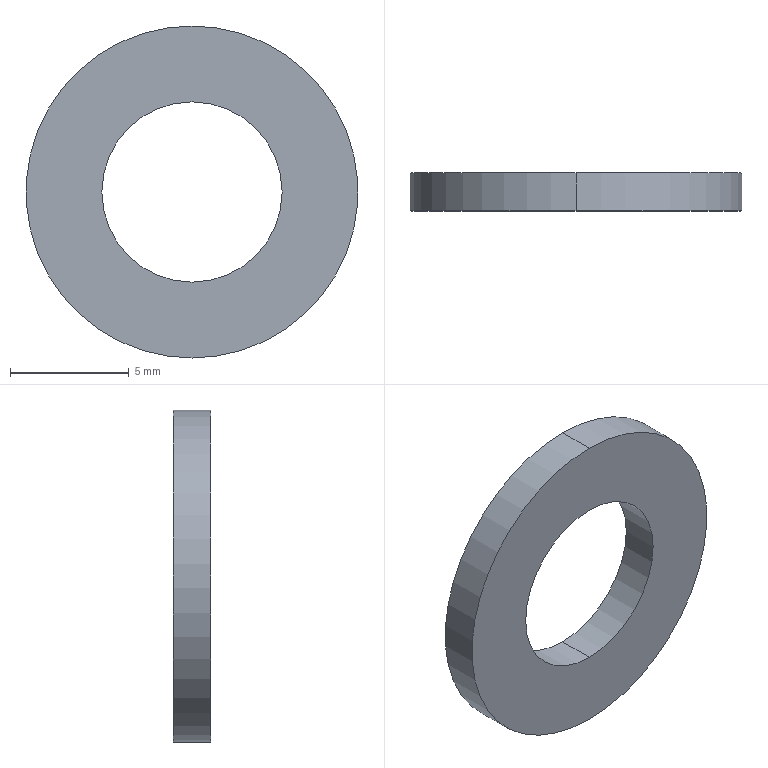Part | SolidWorks | features Revolution 1 | 1 solid | 6 faces | box 14 x 1.6 x 14 mm | volume 173.718 mm3 | cylinder 4 | plane 2 | commonest cylinder face diameters 7.6 x2 14 x2
STEP:
#1=CARTESIAN_POINT('',(0.,-1.6,7.));
#2=VERTEX_POINT('',#1);
#3=CARTESIAN_POINT('',(0.,-1.6,-7.));
#4=VERTEX_POINT('',#3);
#5=CARTESIAN_POINT('',(0.,-1.6,0.));
#6=DIRECTION('',(0.,1.,0.));
#7=DIRECTION('',(0.,0.,1.));
#8=AXIS2_PLACEMENT_3D('',#5,#6,#7);
#9=CIRCLE('',#8,7.);
#10=EDGE_CURVE('',#2,#4,#9,.T.);
#11=ORIENTED_EDGE('',*,*,#10,.T.);
#12=CARTESIAN_POINT('',(0.,0.,-7.));
#13=VERTEX_POINT('',#12);
#14=CARTESIAN_POINT('',(0.,0.,-7.));
#15=DIRECTION('',(0.,1.,0.));
#16=VECTOR('',#15,1000.);
#17=LINE('',#14,#16);
#18=EDGE_CURVE('',#4,#13,#17,.T.);
#19=ORIENTED_EDGE('',*,*,#18,.T.);
#20=CARTESIAN_POINT('',(0.,0.,7.));
#21=VERTEX_POINT('',#20);
#22=CARTESIAN_POINT('',(0.,0.,0.));
#23=DIRECTION('',(0.,1.,0.));
#24=DIRECTION('',(0.,0.,1.));
#25=AXIS2_PLACEMENT_3D('',#22,#23,#24);
#26=CIRCLE('',#25,7.);
#27=EDGE_CURVE('',#21,#13,#26,.T.);
#28=ORIENTED_EDGE('',*,*,#27,.F.);
#29=CARTESIAN_POINT('',(0.,0.,7.));
#30=DIRECTION('',(0.,1.,0.));
#31=VECTOR('',#30,1000.);
#32=LINE('',#29,#31);
#33=EDGE_CURVE('',#2,#21,#32,.T.);
#34=ORIENTED_EDGE('',*,*,#33,.F.);
#35=EDGE_LOOP('',(#11,#19,#28,#34));
#36=FACE_OUTER_BOUND('',#35,.T.);
#37=CARTESIAN_POINT('',(0.,0.,0.));
#38=DIRECTION('',(0.,1.,0.));
#39=DIRECTION('',(0.,0.,1.));
#40=AXIS2_PLACEMENT_3D('',#37,#38,#39);
#41=CYLINDRICAL_SURFACE('',#40,7.);
#42=ADVANCED_FACE('',(#36),#41,.T.);
#43=CARTESIAN_POINT('',(0.,-1.6,-3.8));
#44=VERTEX_POINT('',#43);
#45=CARTESIAN_POINT('',(0.,-1.6,3.8));
#46=VERTEX_POINT('',#45);
#47=CARTESIAN_POINT('',(0.,-1.6,0.));
#48=DIRECTION('',(0.,1.,0.));
#49=DIRECTION('',(0.,0.,1.));
#50=AXIS2_PLACEMENT_3D('',#47,#48,#49);
#51=CIRCLE('',#50,3.8);
#52=EDGE_CURVE('',#44,#46,#51,.T.);
#53=ORIENTED_EDGE('',*,*,#52,.F.);
#54=CARTESIAN_POINT('',(0.,0.,-3.8));
#55=VERTEX_POINT('',#54);
#56=CARTESIAN_POINT('',(0.,0.,-3.8));
#57=DIRECTION('',(0.,1.,0.));
#58=VECTOR('',#57,1000.);
#59=LINE('',#56,#58);
#60=EDGE_CURVE('',#44,#55,#59,.T.);
#61=ORIENTED_EDGE('',*,*,#60,.T.);
#62=CARTESIAN_POINT('',(0.,0.,3.8));
#63=VERTEX_POINT('',#62);
#64=CARTESIAN_POINT('',(0.,0.,0.));
#65=DIRECTION('',(0.,1.,0.));
#66=DIRECTION('',(0.,0.,1.));
#67=AXIS2_PLACEMENT_3D('',#64,#65,#66);
#68=CIRCLE('',#67,3.8);
#69=EDGE_CURVE('',#55,#63,#68,.T.);
#70=ORIENTED_EDGE('',*,*,#69,.T.);
#71=CARTESIAN_POINT('',(0.,0.,3.8));
#72=DIRECTION('',(0.,1.,0.));
#73=VECTOR('',#72,1000.);
#74=LINE('',#71,#73);
#75=EDGE_CURVE('',#46,#63,#74,.T.);
#76=ORIENTED_EDGE('',*,*,#75,.F.);
#77=EDGE_LOOP('',(#53,#61,#70,#76));
#78=FACE_OUTER_BOUND('',#77,.T.);
#79=CARTESIAN_POINT('',(0.,0.,0.));
#80=DIRECTION('',(0.,1.,0.));
#81=DIRECTION('',(0.,0.,1.));
#82=AXIS2_PLACEMENT_3D('',#79,#80,#81);
#83=CYLINDRICAL_SURFACE('',#82,3.8);
#84=ADVANCED_FACE('',(#78),#83,.F.);
#85=ORIENTED_EDGE('',*,*,#60,.F.);
#86=CARTESIAN_POINT('',(0.,-1.6,0.));
#87=DIRECTION('',(0.,1.,0.));
#88=DIRECTION('',(0.,0.,1.));
#89=AXIS2_PLACEMENT_3D('',#86,#87,#88);
#90=CIRCLE('',#89,3.8);
#91=EDGE_CURVE('',#46,#44,#90,.T.);
#92=ORIENTED_EDGE('',*,*,#91,.F.);
#93=ORIENTED_EDGE('',*,*,#75,.T.);
#94=CARTESIAN_POINT('',(0.,0.,0.));
#95=DIRECTION('',(0.,1.,0.));
#96=DIRECTION('',(0.,0.,1.));
#97=AXIS2_PLACEMENT_3D('',#94,#95,#96);
#98=CIRCLE('',#97,3.8);
#99=EDGE_CURVE('',#63,#55,#98,.T.);
#100=ORIENTED_EDGE('',*,*,#99,.T.);
#101=EDGE_LOOP('',(#85,#92,#93,#100));
#102=FACE_OUTER_BOUND('',#101,.T.);
#103=CARTESIAN_POINT('',(0.,0.,0.));
#104=DIRECTION('',(0.,1.,0.));
#105=DIRECTION('',(0.,0.,1.));
#106=AXIS2_PLACEMENT_3D('',#103,#104,#105);
#107=CYLINDRICAL_SURFACE('',#106,3.8);
#108=ADVANCED_FACE('',(#102),#107,.F.);
#109=ORIENTED_EDGE('',*,*,#27,.T.);
#110=CARTESIAN_POINT('',(0.,0.,0.));
#111=DIRECTION('',(0.,1.,0.));
#112=DIRECTION('',(0.,0.,1.));
#113=AXIS2_PLACEMENT_3D('',#110,#111,#112);
#114=CIRCLE('',#113,7.);
#115=EDGE_CURVE('',#13,#21,#114,.T.);
#116=ORIENTED_EDGE('',*,*,#115,.T.);
#117=EDGE_LOOP('',(#109,#116));
#118=FACE_OUTER_BOUND('',#117,.T.);
#119=ORIENTED_EDGE('',*,*,#99,.F.);
#120=ORIENTED_EDGE('',*,*,#69,.F.);
#121=EDGE_LOOP('',(#119,#120));
#122=FACE_BOUND('',#121,.T.);
#123=CARTESIAN_POINT('',(3.8,0.,0.));
#124=DIRECTION('',(0.,1.,0.));
#125=DIRECTION('',(0.,0.,1.));
#126=AXIS2_PLACEMENT_3D('',#123,#124,#125);
#127=PLANE('',#126);
#128=ADVANCED_FACE('',(#118,#122),#127,.T.);
#129=ORIENTED_EDGE('',*,*,#18,.F.);
#130=CARTESIAN_POINT('',(0.,-1.6,0.));
#131=DIRECTION('',(0.,1.,0.));
#132=DIRECTION('',(0.,0.,1.));
#133=AXIS2_PLACEMENT_3D('',#130,#131,#132);
#134=CIRCLE('',#133,7.);
#135=EDGE_CURVE('',#4,#2,#134,.T.);
#136=ORIENTED_EDGE('',*,*,#135,.T.);
#137=ORIENTED_EDGE('',*,*,#33,.T.);
#138=ORIENTED_EDGE('',*,*,#115,.F.);
#139=EDGE_LOOP('',(#129,#136,#137,#138));
#140=FACE_OUTER_BOUND('',#139,.T.);
#141=CARTESIAN_POINT('',(0.,0.,0.));
#142=DIRECTION('',(0.,1.,0.));
#143=DIRECTION('',(0.,0.,1.));
#144=AXIS2_PLACEMENT_3D('',#141,#142,#143);
#145=CYLINDRICAL_SURFACE('',#144,7.);
#146=ADVANCED_FACE('',(#140),#145,.T.);
#147=ORIENTED_EDGE('',*,*,#91,.T.);
#148=ORIENTED_EDGE('',*,*,#52,.T.);
#149=EDGE_LOOP('',(#147,#148));
#150=FACE_BOUND('',#149,.T.);
#151=ORIENTED_EDGE('',*,*,#10,.F.);
#152=ORIENTED_EDGE('',*,*,#135,.F.);
#153=EDGE_LOOP('',(#151,#152));
#154=FACE_OUTER_BOUND('',#153,.T.);
#155=CARTESIAN_POINT('',(3.8,-1.6,0.));
#156=DIRECTION('',(0.,-1.,0.));
#157=DIRECTION('',(0.,0.,-1.));
#158=AXIS2_PLACEMENT_3D('',#155,#156,#157);
#159=PLANE('',#158);
#160=ADVANCED_FACE('',(#150,#154),#159,.T.);
#161=CLOSED_SHELL('',(#42,#84,#108,#128,#146,#160));
#162=MANIFOLD_SOLID_BREP('',#161);
#163=CARTESIAN_POINT('',(0.,0.,0.));
#164=DIRECTION('',(0.,0.,1.));
#165=DIRECTION('',(1.,0.,0.));
#166=AXIS2_PLACEMENT_3D('',#163,#164,#165);
#167=(LENGTH_UNIT()NAMED_UNIT(*)SI_UNIT(.MILLI.,.METRE.));
#168=UNCERTAINTY_MEASURE_WITH_UNIT(LENGTH_MEASURE(0.00001),#167,'','');
#169=(NAMED_UNIT(*)PLANE_ANGLE_UNIT()SI_UNIT($,.RADIAN.));
#170=(NAMED_UNIT(*)SI_UNIT($,.STERADIAN.)SOLID_ANGLE_UNIT());
#171=(GEOMETRIC_REPRESENTATION_CONTEXT(3)GLOBAL_UNCERTAINTY_ASSIGNED_CONTEXT((#168))GLOBAL_UNIT_ASSIGNED_CONTEXT((#167,#169,#170))REPRESENTATION_CONTEXT('',''));
#172=ADVANCED_BREP_SHAPE_REPRESENTATION('',(#162,#166),#171);